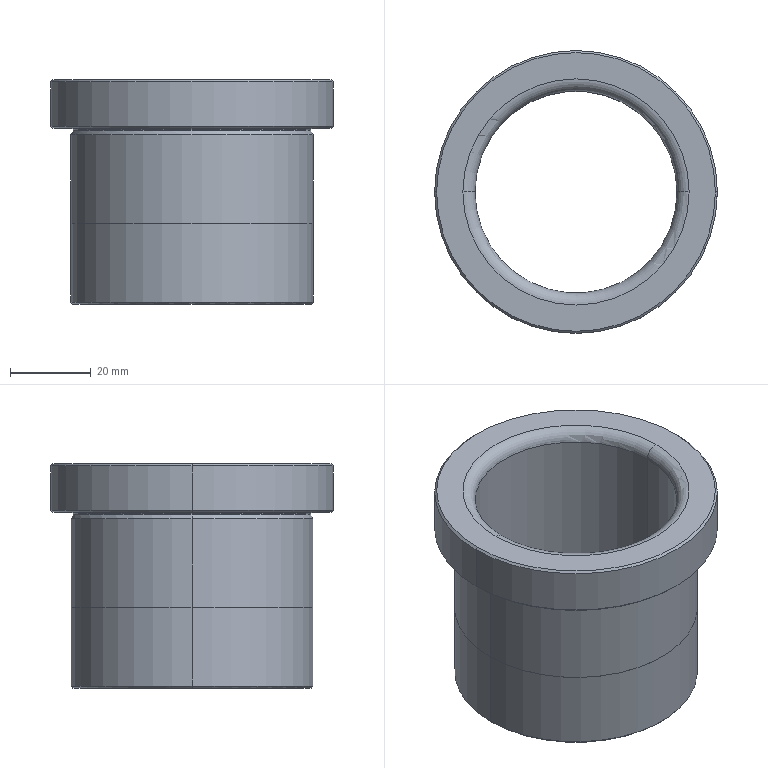Part | STEP file | Bucha B - B50056 | 1 solid | 28 faces | box 70 x 70 x 55.5 mm | volume 59351 mm3 | torus 8 | cone 8 | cylinder 8 | plane 4 | commonest cylinder face diameters 50 x2 59.98 x2 60 x2 70 x2